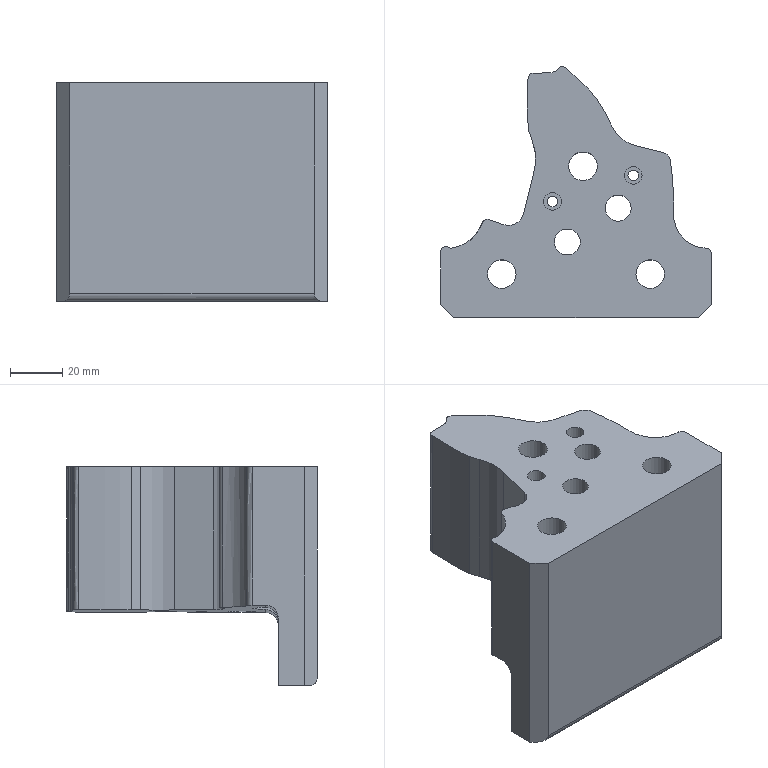Part | NX | features solid 2 | 1 solid | 63 faces | box 104 x 96.282 x 84 mm | volume 327041 mm3 | cylinder 24 | plane 21 | spline 18 | commonest cylinder face diameters 10 x6 11 x5 17 x3 4.1 x2 6 x2 6.8 x2